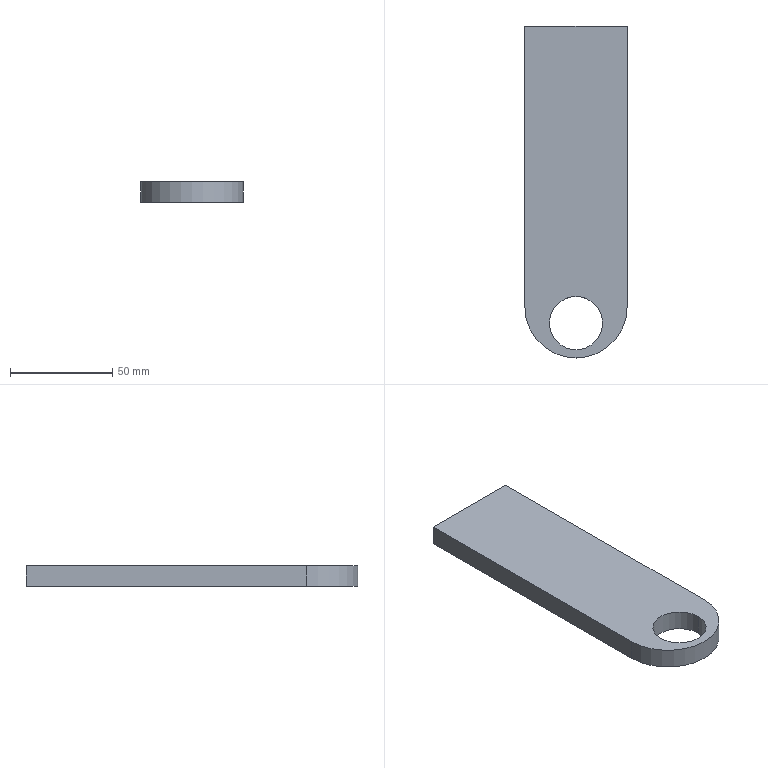Part | SolidWorks | features Extrusion 1, ICE 1 | 1 solid | 8 faces | box 50 x 162 x 10 mm | volume 73008 mm3 | plane 5 | cylinder 3 | commonest cylinder face diameters 26 x2 50 x1
STEP:
#1=CARTESIAN_POINT('',(-13.,-8.,0.));
#2=VERTEX_POINT('',#1);
#3=CARTESIAN_POINT('',(13.,-8.,0.));
#4=VERTEX_POINT('',#3);
#5=CARTESIAN_POINT('',(0.,-8.,0.));
#6=DIRECTION('',(0.,0.,1.));
#7=DIRECTION('',(1.,0.,0.));
#8=AXIS2_PLACEMENT_3D('',#5,#6,#7);
#9=CIRCLE('',#8,13.);
#10=EDGE_CURVE('',#2,#4,#9,.T.);
#11=ORIENTED_EDGE('',*,*,#10,.F.);
#12=CARTESIAN_POINT('',(-13.,-8.,10.));
#13=VERTEX_POINT('',#12);
#14=CARTESIAN_POINT('',(-13.,-8.,0.));
#15=DIRECTION('',(0.,0.,1.));
#16=VECTOR('',#15,1000.);
#17=LINE('',#14,#16);
#18=EDGE_CURVE('',#2,#13,#17,.T.);
#19=ORIENTED_EDGE('',*,*,#18,.T.);
#20=CARTESIAN_POINT('',(13.,-8.,10.));
#21=VERTEX_POINT('',#20);
#22=CARTESIAN_POINT('',(0.,-8.,10.));
#23=DIRECTION('',(0.,0.,1.));
#24=DIRECTION('',(1.,0.,0.));
#25=AXIS2_PLACEMENT_3D('',#22,#23,#24);
#26=CIRCLE('',#25,13.);
#27=EDGE_CURVE('',#13,#21,#26,.T.);
#28=ORIENTED_EDGE('',*,*,#27,.T.);
#29=CARTESIAN_POINT('',(13.,-8.,0.));
#30=DIRECTION('',(0.,0.,1.));
#31=VECTOR('',#30,1000.);
#32=LINE('',#29,#31);
#33=EDGE_CURVE('',#4,#21,#32,.T.);
#34=ORIENTED_EDGE('',*,*,#33,.F.);
#35=EDGE_LOOP('',(#11,#19,#28,#34));
#36=FACE_OUTER_BOUND('',#35,.T.);
#37=CARTESIAN_POINT('',(0.,-8.,0.));
#38=DIRECTION('',(0.,0.,1.));
#39=DIRECTION('',(1.,0.,0.));
#40=AXIS2_PLACEMENT_3D('',#37,#38,#39);
#41=CYLINDRICAL_SURFACE('',#40,13.);
#42=ADVANCED_FACE('',(#36),#41,.F.);
#43=CARTESIAN_POINT('',(-25.,0.,0.));
#44=VERTEX_POINT('',#43);
#45=CARTESIAN_POINT('',(25.,0.,0.));
#46=VERTEX_POINT('',#45);
#47=CARTESIAN_POINT('',(0.,0.,0.));
#48=DIRECTION('',(0.,0.,1.));
#49=DIRECTION('',(1.,0.,0.));
#50=AXIS2_PLACEMENT_3D('',#47,#48,#49);
#51=CIRCLE('',#50,25.);
#52=EDGE_CURVE('',#44,#46,#51,.T.);
#53=ORIENTED_EDGE('',*,*,#52,.T.);
#54=CARTESIAN_POINT('',(25.,0.,10.));
#55=VERTEX_POINT('',#54);
#56=CARTESIAN_POINT('',(25.,0.,10.));
#57=DIRECTION('',(0.,0.,-1.));
#58=VECTOR('',#57,1000.);
#59=LINE('',#56,#58);
#60=EDGE_CURVE('',#55,#46,#59,.T.);
#61=ORIENTED_EDGE('',*,*,#60,.F.);
#62=CARTESIAN_POINT('',(-25.,0.,10.));
#63=VERTEX_POINT('',#62);
#64=CARTESIAN_POINT('',(0.,0.,10.));
#65=DIRECTION('',(0.,0.,1.));
#66=DIRECTION('',(1.,0.,0.));
#67=AXIS2_PLACEMENT_3D('',#64,#65,#66);
#68=CIRCLE('',#67,25.);
#69=EDGE_CURVE('',#63,#55,#68,.T.);
#70=ORIENTED_EDGE('',*,*,#69,.F.);
#71=CARTESIAN_POINT('',(-25.,0.,10.));
#72=DIRECTION('',(0.,0.,-1.));
#73=VECTOR('',#72,1000.);
#74=LINE('',#71,#73);
#75=EDGE_CURVE('',#63,#44,#74,.T.);
#76=ORIENTED_EDGE('',*,*,#75,.T.);
#77=EDGE_LOOP('',(#53,#61,#70,#76));
#78=FACE_OUTER_BOUND('',#77,.T.);
#79=CARTESIAN_POINT('',(0.,0.,10.));
#80=DIRECTION('',(0.,0.,-1.));
#81=DIRECTION('',(-1.,0.,0.));
#82=AXIS2_PLACEMENT_3D('',#79,#80,#81);
#83=CYLINDRICAL_SURFACE('',#82,25.);
#84=ADVANCED_FACE('',(#78),#83,.T.);
#85=CARTESIAN_POINT('',(25.,137.,0.));
#86=VERTEX_POINT('',#85);
#87=CARTESIAN_POINT('',(25.,137.,0.));
#88=DIRECTION('',(0.,1.,0.));
#89=VECTOR('',#88,1000.);
#90=LINE('',#87,#89);
#91=EDGE_CURVE('',#46,#86,#90,.T.);
#92=ORIENTED_EDGE('',*,*,#91,.T.);
#93=CARTESIAN_POINT('',(25.,137.,10.));
#94=VERTEX_POINT('',#93);
#95=CARTESIAN_POINT('',(25.,137.,10.));
#96=DIRECTION('',(0.,0.,-1.));
#97=VECTOR('',#96,1000.);
#98=LINE('',#95,#97);
#99=EDGE_CURVE('',#94,#86,#98,.T.);
#100=ORIENTED_EDGE('',*,*,#99,.F.);
#101=CARTESIAN_POINT('',(25.,137.,10.));
#102=DIRECTION('',(0.,1.,0.));
#103=VECTOR('',#102,1000.);
#104=LINE('',#101,#103);
#105=EDGE_CURVE('',#55,#94,#104,.T.);
#106=ORIENTED_EDGE('',*,*,#105,.F.);
#107=ORIENTED_EDGE('',*,*,#60,.T.);
#108=EDGE_LOOP('',(#92,#100,#106,#107));
#109=FACE_OUTER_BOUND('',#108,.T.);
#110=CARTESIAN_POINT('',(25.,137.,10.));
#111=DIRECTION('',(-1.,0.,0.));
#112=DIRECTION('',(0.,-1.,0.));
#113=AXIS2_PLACEMENT_3D('',#110,#111,#112);
#114=PLANE('',#113);
#115=ADVANCED_FACE('',(#109),#114,.F.);
#116=CARTESIAN_POINT('',(-25.,137.,0.));
#117=VERTEX_POINT('',#116);
#118=CARTESIAN_POINT('',(-25.,137.,0.));
#119=DIRECTION('',(-1.,0.,0.));
#120=VECTOR('',#119,1000.);
#121=LINE('',#118,#120);
#122=EDGE_CURVE('',#86,#117,#121,.T.);
#123=ORIENTED_EDGE('',*,*,#122,.T.);
#124=CARTESIAN_POINT('',(-25.,137.,10.));
#125=VERTEX_POINT('',#124);
#126=CARTESIAN_POINT('',(-25.,137.,10.));
#127=DIRECTION('',(0.,0.,-1.));
#128=VECTOR('',#127,1000.);
#129=LINE('',#126,#128);
#130=EDGE_CURVE('',#125,#117,#129,.T.);
#131=ORIENTED_EDGE('',*,*,#130,.F.);
#132=CARTESIAN_POINT('',(-25.,137.,10.));
#133=DIRECTION('',(-1.,0.,0.));
#134=VECTOR('',#133,1000.);
#135=LINE('',#132,#134);
#136=EDGE_CURVE('',#94,#125,#135,.T.);
#137=ORIENTED_EDGE('',*,*,#136,.F.);
#138=ORIENTED_EDGE('',*,*,#99,.T.);
#139=EDGE_LOOP('',(#123,#131,#137,#138));
#140=FACE_OUTER_BOUND('',#139,.T.);
#141=CARTESIAN_POINT('',(-25.,137.,10.));
#142=DIRECTION('',(0.,-1.,0.));
#143=DIRECTION('',(0.,0.,-1.));
#144=AXIS2_PLACEMENT_3D('',#141,#142,#143);
#145=PLANE('',#144);
#146=ADVANCED_FACE('',(#140),#145,.F.);
#147=CARTESIAN_POINT('',(-25.,0.,0.));
#148=DIRECTION('',(0.,-1.,0.));
#149=VECTOR('',#148,1000.);
#150=LINE('',#147,#149);
#151=EDGE_CURVE('',#117,#44,#150,.T.);
#152=ORIENTED_EDGE('',*,*,#151,.T.);
#153=ORIENTED_EDGE('',*,*,#75,.F.);
#154=CARTESIAN_POINT('',(-25.,0.,10.));
#155=DIRECTION('',(0.,-1.,0.));
#156=VECTOR('',#155,1000.);
#157=LINE('',#154,#156);
#158=EDGE_CURVE('',#125,#63,#157,.T.);
#159=ORIENTED_EDGE('',*,*,#158,.F.);
#160=ORIENTED_EDGE('',*,*,#130,.T.);
#161=EDGE_LOOP('',(#152,#153,#159,#160));
#162=FACE_OUTER_BOUND('',#161,.T.);
#163=CARTESIAN_POINT('',(-25.,0.,10.));
#164=DIRECTION('',(1.,0.,0.));
#165=DIRECTION('',(0.,1.,0.));
#166=AXIS2_PLACEMENT_3D('',#163,#164,#165);
#167=PLANE('',#166);
#168=ADVANCED_FACE('',(#162),#167,.F.);
#169=CARTESIAN_POINT('',(0.,-8.,10.));
#170=DIRECTION('',(0.,0.,1.));
#171=DIRECTION('',(1.,0.,0.));
#172=AXIS2_PLACEMENT_3D('',#169,#170,#171);
#173=CIRCLE('',#172,13.);
#174=EDGE_CURVE('',#21,#13,#173,.T.);
#175=ORIENTED_EDGE('',*,*,#174,.F.);
#176=ORIENTED_EDGE('',*,*,#27,.F.);
#177=EDGE_LOOP('',(#175,#176));
#178=FACE_BOUND('',#177,.T.);
#179=ORIENTED_EDGE('',*,*,#69,.T.);
#180=ORIENTED_EDGE('',*,*,#105,.T.);
#181=ORIENTED_EDGE('',*,*,#136,.T.);
#182=ORIENTED_EDGE('',*,*,#158,.T.);
#183=EDGE_LOOP('',(#179,#180,#181,#182));
#184=FACE_OUTER_BOUND('',#183,.T.);
#185=CARTESIAN_POINT('',(0.,0.,10.));
#186=DIRECTION('',(0.,0.,1.));
#187=DIRECTION('',(1.,0.,0.));
#188=AXIS2_PLACEMENT_3D('',#185,#186,#187);
#189=PLANE('',#188);
#190=ADVANCED_FACE('',(#178,#184),#189,.T.);
#191=CARTESIAN_POINT('',(0.,-8.,0.));
#192=DIRECTION('',(0.,0.,1.));
#193=DIRECTION('',(1.,0.,0.));
#194=AXIS2_PLACEMENT_3D('',#191,#192,#193);
#195=CIRCLE('',#194,13.);
#196=EDGE_CURVE('',#4,#2,#195,.T.);
#197=ORIENTED_EDGE('',*,*,#196,.T.);
#198=ORIENTED_EDGE('',*,*,#10,.T.);
#199=EDGE_LOOP('',(#197,#198));
#200=FACE_BOUND('',#199,.T.);
#201=ORIENTED_EDGE('',*,*,#52,.F.);
#202=ORIENTED_EDGE('',*,*,#151,.F.);
#203=ORIENTED_EDGE('',*,*,#122,.F.);
#204=ORIENTED_EDGE('',*,*,#91,.F.);
#205=EDGE_LOOP('',(#201,#202,#203,#204));
#206=FACE_OUTER_BOUND('',#205,.T.);
#207=CARTESIAN_POINT('',(0.,0.,0.));
#208=DIRECTION('',(0.,0.,1.));
#209=DIRECTION('',(1.,0.,0.));
#210=AXIS2_PLACEMENT_3D('',#207,#208,#209);
#211=PLANE('',#210);
#212=ADVANCED_FACE('',(#200,#206),#211,.F.);
#213=ORIENTED_EDGE('',*,*,#18,.F.);
#214=ORIENTED_EDGE('',*,*,#196,.F.);
#215=ORIENTED_EDGE('',*,*,#33,.T.);
#216=ORIENTED_EDGE('',*,*,#174,.T.);
#217=EDGE_LOOP('',(#213,#214,#215,#216));
#218=FACE_OUTER_BOUND('',#217,.T.);
#219=CARTESIAN_POINT('',(0.,-8.,0.));
#220=DIRECTION('',(0.,0.,1.));
#221=DIRECTION('',(1.,0.,0.));
#222=AXIS2_PLACEMENT_3D('',#219,#220,#221);
#223=CYLINDRICAL_SURFACE('',#222,13.);
#224=ADVANCED_FACE('',(#218),#223,.F.);
#225=CLOSED_SHELL('',(#42,#84,#115,#146,#168,#190,#212,#224));
#226=MANIFOLD_SOLID_BREP('',#225);
#227=CARTESIAN_POINT('',(0.,0.,0.));
#228=DIRECTION('',(0.,0.,1.));
#229=DIRECTION('',(1.,0.,0.));
#230=AXIS2_PLACEMENT_3D('',#227,#228,#229);
#231=(LENGTH_UNIT()NAMED_UNIT(*)SI_UNIT(.MILLI.,.METRE.));
#232=UNCERTAINTY_MEASURE_WITH_UNIT(LENGTH_MEASURE(0.00001),#231,'','');
#233=(NAMED_UNIT(*)PLANE_ANGLE_UNIT()SI_UNIT($,.RADIAN.));
#234=(NAMED_UNIT(*)SI_UNIT($,.STERADIAN.)SOLID_ANGLE_UNIT());
#235=(GEOMETRIC_REPRESENTATION_CONTEXT(3)GLOBAL_UNCERTAINTY_ASSIGNED_CONTEXT((#232))GLOBAL_UNIT_ASSIGNED_CONTEXT((#231,#233,#234))REPRESENTATION_CONTEXT('',''));
#236=ADVANCED_BREP_SHAPE_REPRESENTATION('',(#226,#230),#235);